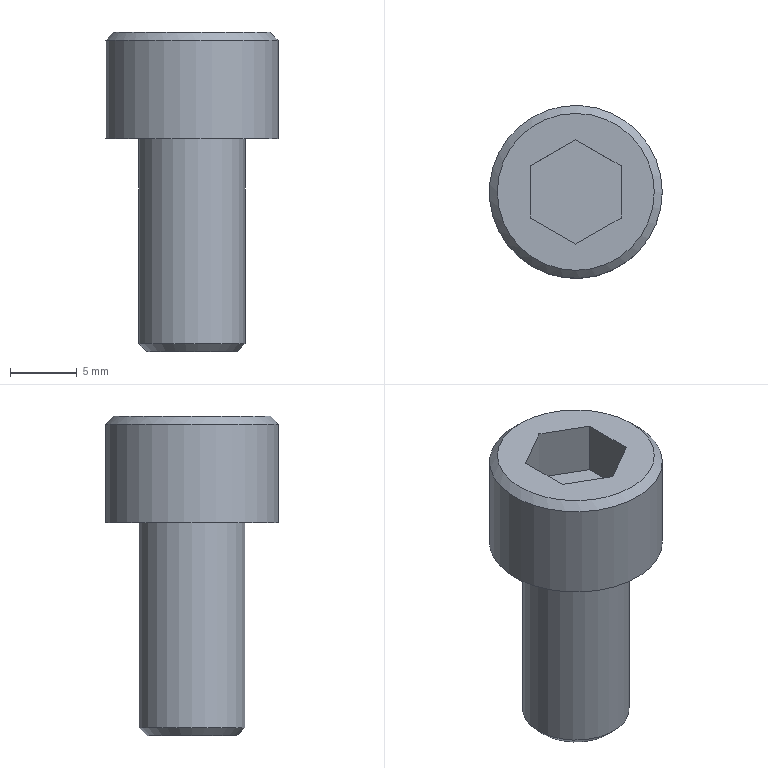Part | NX | features M8.00-50.00 2 | 1 solid | 14 faces | box 13 x 13 x 24 mm | volume 1695 mm3 | plane 10 | cylinder 2 | cone 2 | commonest cylinder face diameters 8 x1 13 x1
STEP:
#1=CARTESIAN_POINT('',(169.4,-50.,-42.));
#2=VERTEX_POINT('',#1);
#3=CARTESIAN_POINT('',(163.5,-50.,-42.));
#4=DIRECTION('',(0.,0.,1.));
#5=DIRECTION('',(1.,0.,0.));
#6=AXIS2_PLACEMENT_3D('',#3,#4,#5);
#7=CIRCLE('',#6,5.9);
#8=EDGE_CURVE('',#2,#2,#7,.T.);
#9=ORIENTED_EDGE('',*,*,#8,.T.);
#10=EDGE_LOOP('',(#9));
#11=FACE_BOUND('',#10,.T.);
#12=CARTESIAN_POINT('',(160.1,-48.037,-42.));
#13=VERTEX_POINT('',#12);
#14=CARTESIAN_POINT('',(160.1,-51.963,-42.));
#15=VERTEX_POINT('',#14);
#16=CARTESIAN_POINT('',(160.1,-48.037,-42.));
#17=DIRECTION('',(0.,-1.,0.));
#18=VECTOR('',#17,1000.);
#19=LINE('',#16,#18);
#20=EDGE_CURVE('',#13,#15,#19,.T.);
#21=ORIENTED_EDGE('',*,*,#20,.F.);
#22=CARTESIAN_POINT('',(163.5,-46.074,-42.));
#23=VERTEX_POINT('',#22);
#24=CARTESIAN_POINT('',(163.5,-46.074,-42.));
#25=DIRECTION('',(-0.866,-0.5,0.));
#26=VECTOR('',#25,1000.);
#27=LINE('',#24,#26);
#28=EDGE_CURVE('',#23,#13,#27,.T.);
#29=ORIENTED_EDGE('',*,*,#28,.F.);
#30=CARTESIAN_POINT('',(166.9,-48.037,-42.));
#31=VERTEX_POINT('',#30);
#32=CARTESIAN_POINT('',(166.9,-48.037,-42.));
#33=DIRECTION('',(-0.866,0.5,0.));
#34=VECTOR('',#33,1000.);
#35=LINE('',#32,#34);
#36=EDGE_CURVE('',#31,#23,#35,.T.);
#37=ORIENTED_EDGE('',*,*,#36,.F.);
#38=CARTESIAN_POINT('',(166.9,-51.963,-42.));
#39=VERTEX_POINT('',#38);
#40=CARTESIAN_POINT('',(166.9,-51.963,-42.));
#41=DIRECTION('',(0.,1.,0.));
#42=VECTOR('',#41,1000.);
#43=LINE('',#40,#42);
#44=EDGE_CURVE('',#39,#31,#43,.T.);
#45=ORIENTED_EDGE('',*,*,#44,.F.);
#46=CARTESIAN_POINT('',(163.5,-53.926,-42.));
#47=VERTEX_POINT('',#46);
#48=CARTESIAN_POINT('',(163.5,-53.926,-42.));
#49=DIRECTION('',(0.866,0.5,0.));
#50=VECTOR('',#49,1000.);
#51=LINE('',#48,#50);
#52=EDGE_CURVE('',#47,#39,#51,.T.);
#53=ORIENTED_EDGE('',*,*,#52,.F.);
#54=CARTESIAN_POINT('',(160.1,-51.963,-42.));
#55=DIRECTION('',(0.866,-0.5,0.));
#56=VECTOR('',#55,1000.);
#57=LINE('',#54,#56);
#58=EDGE_CURVE('',#15,#47,#57,.T.);
#59=ORIENTED_EDGE('',*,*,#58,.F.);
#60=EDGE_LOOP('',(#21,#29,#37,#45,#53,#59));
#61=FACE_BOUND('',#60,.T.);
#62=CARTESIAN_POINT('',(163.5,-50.,-42.));
#63=DIRECTION('',(0.,0.,1.));
#64=DIRECTION('',(1.,0.,0.));
#65=AXIS2_PLACEMENT_3D('',#62,#63,#64);
#66=PLANE('',#65);
#67=ADVANCED_FACE('',(#11,#61),#66,.T.);
#68=CARTESIAN_POINT('',(167.5,-50.,-50.));
#69=VERTEX_POINT('',#68);
#70=CARTESIAN_POINT('',(163.5,-50.,-50.));
#71=DIRECTION('',(0.,0.,-1.));
#72=DIRECTION('',(1.,0.,0.));
#73=AXIS2_PLACEMENT_3D('',#70,#71,#72);
#74=CIRCLE('',#73,4.);
#75=EDGE_CURVE('',#69,#69,#74,.T.);
#76=ORIENTED_EDGE('',*,*,#75,.F.);
#77=EDGE_LOOP('',(#76));
#78=FACE_BOUND('',#77,.T.);
#79=CARTESIAN_POINT('',(170.,-50.,-50.));
#80=VERTEX_POINT('',#79);
#81=CARTESIAN_POINT('',(163.5,-50.,-50.));
#82=DIRECTION('',(0.,0.,1.));
#83=DIRECTION('',(1.,0.,0.));
#84=AXIS2_PLACEMENT_3D('',#81,#82,#83);
#85=CIRCLE('',#84,6.5);
#86=EDGE_CURVE('',#80,#80,#85,.T.);
#87=ORIENTED_EDGE('',*,*,#86,.F.);
#88=EDGE_LOOP('',(#87));
#89=FACE_BOUND('',#88,.T.);
#90=CARTESIAN_POINT('',(163.5,-50.,-50.));
#91=DIRECTION('',(0.,0.,-1.));
#92=DIRECTION('',(-1.,0.,0.));
#93=AXIS2_PLACEMENT_3D('',#90,#91,#92);
#94=PLANE('',#93);
#95=ADVANCED_FACE('',(#78,#89),#94,.T.);
#96=CARTESIAN_POINT('',(170.,-50.,-42.6));
#97=VERTEX_POINT('',#96);
#98=CARTESIAN_POINT('',(163.5,-50.,-42.6));
#99=DIRECTION('',(0.,0.,1.));
#100=DIRECTION('',(1.,0.,0.));
#101=AXIS2_PLACEMENT_3D('',#98,#99,#100);
#102=CIRCLE('',#101,6.5);
#103=EDGE_CURVE('',#97,#97,#102,.F.);
#104=ORIENTED_EDGE('',*,*,#103,.T.);
#105=EDGE_LOOP('',(#104));
#106=FACE_BOUND('',#105,.T.);
#107=ORIENTED_EDGE('',*,*,#86,.T.);
#108=EDGE_LOOP('',(#107));
#109=FACE_BOUND('',#108,.T.);
#110=CARTESIAN_POINT('',(163.5,-50.,-50.));
#111=DIRECTION('',(0.,0.,1.));
#112=DIRECTION('',(1.,0.,0.));
#113=AXIS2_PLACEMENT_3D('',#110,#111,#112);
#114=CYLINDRICAL_SURFACE('',#113,6.5);
#115=ADVANCED_FACE('',(#106,#109),#114,.T.);
#116=CARTESIAN_POINT('',(160.1,-50.,-66.));
#117=VERTEX_POINT('',#116);
#118=CARTESIAN_POINT('',(163.5,-50.,-66.));
#119=DIRECTION('',(0.,0.,-1.));
#120=DIRECTION('',(-1.,0.,0.));
#121=AXIS2_PLACEMENT_3D('',#118,#119,#120);
#122=CIRCLE('',#121,3.4);
#123=EDGE_CURVE('',#117,#117,#122,.T.);
#124=ORIENTED_EDGE('',*,*,#123,.T.);
#125=EDGE_LOOP('',(#124));
#126=FACE_BOUND('',#125,.T.);
#127=CARTESIAN_POINT('',(163.5,-50.,-66.));
#128=DIRECTION('',(0.,0.,-1.));
#129=DIRECTION('',(-1.,0.,0.));
#130=AXIS2_PLACEMENT_3D('',#127,#128,#129);
#131=PLANE('',#130);
#132=ADVANCED_FACE('',(#126),#131,.T.);
#133=CARTESIAN_POINT('',(159.5,-50.,-65.4));
#134=VERTEX_POINT('',#133);
#135=CARTESIAN_POINT('',(163.5,-50.,-65.4));
#136=DIRECTION('',(0.,0.,-1.));
#137=DIRECTION('',(-1.,0.,0.));
#138=AXIS2_PLACEMENT_3D('',#135,#136,#137);
#139=CIRCLE('',#138,4.);
#140=EDGE_CURVE('',#134,#134,#139,.F.);
#141=ORIENTED_EDGE('',*,*,#140,.T.);
#142=EDGE_LOOP('',(#141));
#143=FACE_BOUND('',#142,.T.);
#144=ORIENTED_EDGE('',*,*,#75,.T.);
#145=EDGE_LOOP('',(#144));
#146=FACE_BOUND('',#145,.T.);
#147=CARTESIAN_POINT('',(163.5,-50.,-24.5));
#148=DIRECTION('',(0.,0.,-1.));
#149=DIRECTION('',(1.,0.,0.));
#150=AXIS2_PLACEMENT_3D('',#147,#148,#149);
#151=CYLINDRICAL_SURFACE('',#150,4.);
#152=ADVANCED_FACE('',(#143,#146),#151,.T.);
#153=ORIENTED_EDGE('',*,*,#58,.T.);
#154=CARTESIAN_POINT('',(163.5,-53.926,-46.));
#155=VERTEX_POINT('',#154);
#156=CARTESIAN_POINT('',(163.5,-53.926,-46.));
#157=DIRECTION('',(0.,0.,1.));
#158=VECTOR('',#157,1000.);
#159=LINE('',#156,#158);
#160=EDGE_CURVE('',#47,#155,#159,.F.);
#161=ORIENTED_EDGE('',*,*,#160,.T.);
#162=CARTESIAN_POINT('',(160.1,-51.963,-46.));
#163=VERTEX_POINT('',#162);
#164=CARTESIAN_POINT('',(160.1,-51.963,-46.));
#165=DIRECTION('',(0.866,-0.5,0.));
#166=VECTOR('',#165,1000.);
#167=LINE('',#164,#166);
#168=EDGE_CURVE('',#155,#163,#167,.F.);
#169=ORIENTED_EDGE('',*,*,#168,.T.);
#170=CARTESIAN_POINT('',(160.1,-51.963,-46.));
#171=DIRECTION('',(0.,0.,1.));
#172=VECTOR('',#171,1000.);
#173=LINE('',#170,#172);
#174=EDGE_CURVE('',#15,#163,#173,.F.);
#175=ORIENTED_EDGE('',*,*,#174,.F.);
#176=EDGE_LOOP('',(#153,#161,#169,#175));
#177=FACE_BOUND('',#176,.T.);
#178=CARTESIAN_POINT('',(161.8,-52.944,-44.));
#179=DIRECTION('',(-0.5,-0.866,0.));
#180=DIRECTION('',(0.866,-0.5,0.));
#181=AXIS2_PLACEMENT_3D('',#178,#179,#180);
#182=PLANE('',#181);
#183=ADVANCED_FACE('',(#177),#182,.F.);
#184=ORIENTED_EDGE('',*,*,#20,.T.);
#185=ORIENTED_EDGE('',*,*,#174,.T.);
#186=CARTESIAN_POINT('',(160.1,-48.037,-46.));
#187=VERTEX_POINT('',#186);
#188=CARTESIAN_POINT('',(160.1,-48.037,-46.));
#189=DIRECTION('',(0.,-1.,0.));
#190=VECTOR('',#189,1000.);
#191=LINE('',#188,#190);
#192=EDGE_CURVE('',#163,#187,#191,.F.);
#193=ORIENTED_EDGE('',*,*,#192,.T.);
#194=CARTESIAN_POINT('',(160.1,-48.037,-46.));
#195=DIRECTION('',(0.,0.,1.));
#196=VECTOR('',#195,1000.);
#197=LINE('',#194,#196);
#198=EDGE_CURVE('',#13,#187,#197,.F.);
#199=ORIENTED_EDGE('',*,*,#198,.F.);
#200=EDGE_LOOP('',(#184,#185,#193,#199));
#201=FACE_BOUND('',#200,.T.);
#202=CARTESIAN_POINT('',(160.1,-50.,-44.));
#203=DIRECTION('',(-1.,0.,0.));
#204=DIRECTION('',(0.,0.,1.));
#205=AXIS2_PLACEMENT_3D('',#202,#203,#204);
#206=PLANE('',#205);
#207=ADVANCED_FACE('',(#201),#206,.F.);
#208=ORIENTED_EDGE('',*,*,#28,.T.);
#209=ORIENTED_EDGE('',*,*,#198,.T.);
#210=CARTESIAN_POINT('',(163.5,-46.074,-46.));
#211=VERTEX_POINT('',#210);
#212=CARTESIAN_POINT('',(163.5,-46.074,-46.));
#213=DIRECTION('',(-0.866,-0.5,0.));
#214=VECTOR('',#213,1000.);
#215=LINE('',#212,#214);
#216=EDGE_CURVE('',#187,#211,#215,.F.);
#217=ORIENTED_EDGE('',*,*,#216,.T.);
#218=CARTESIAN_POINT('',(163.5,-46.074,-46.));
#219=DIRECTION('',(0.,0.,1.));
#220=VECTOR('',#219,1000.);
#221=LINE('',#218,#220);
#222=EDGE_CURVE('',#23,#211,#221,.F.);
#223=ORIENTED_EDGE('',*,*,#222,.F.);
#224=EDGE_LOOP('',(#208,#209,#217,#223));
#225=FACE_BOUND('',#224,.T.);
#226=CARTESIAN_POINT('',(161.8,-47.056,-44.));
#227=DIRECTION('',(-0.5,0.866,0.));
#228=DIRECTION('',(-0.866,-0.5,0.));
#229=AXIS2_PLACEMENT_3D('',#226,#227,#228);
#230=PLANE('',#229);
#231=ADVANCED_FACE('',(#225),#230,.F.);
#232=ORIENTED_EDGE('',*,*,#36,.T.);
#233=ORIENTED_EDGE('',*,*,#222,.T.);
#234=CARTESIAN_POINT('',(166.9,-48.037,-46.));
#235=VERTEX_POINT('',#234);
#236=CARTESIAN_POINT('',(166.9,-48.037,-46.));
#237=DIRECTION('',(-0.866,0.5,0.));
#238=VECTOR('',#237,1000.);
#239=LINE('',#236,#238);
#240=EDGE_CURVE('',#211,#235,#239,.F.);
#241=ORIENTED_EDGE('',*,*,#240,.T.);
#242=CARTESIAN_POINT('',(166.9,-48.037,-46.));
#243=DIRECTION('',(0.,0.,1.));
#244=VECTOR('',#243,1000.);
#245=LINE('',#242,#244);
#246=EDGE_CURVE('',#31,#235,#245,.F.);
#247=ORIENTED_EDGE('',*,*,#246,.F.);
#248=EDGE_LOOP('',(#232,#233,#241,#247));
#249=FACE_BOUND('',#248,.T.);
#250=CARTESIAN_POINT('',(165.2,-47.056,-44.));
#251=DIRECTION('',(0.5,0.866,0.));
#252=DIRECTION('',(-0.866,0.5,0.));
#253=AXIS2_PLACEMENT_3D('',#250,#251,#252);
#254=PLANE('',#253);
#255=ADVANCED_FACE('',(#249),#254,.F.);
#256=ORIENTED_EDGE('',*,*,#44,.T.);
#257=ORIENTED_EDGE('',*,*,#246,.T.);
#258=CARTESIAN_POINT('',(166.9,-51.963,-46.));
#259=VERTEX_POINT('',#258);
#260=CARTESIAN_POINT('',(166.9,-51.963,-46.));
#261=DIRECTION('',(0.,1.,0.));
#262=VECTOR('',#261,1000.);
#263=LINE('',#260,#262);
#264=EDGE_CURVE('',#235,#259,#263,.F.);
#265=ORIENTED_EDGE('',*,*,#264,.T.);
#266=CARTESIAN_POINT('',(166.9,-51.963,-46.));
#267=DIRECTION('',(0.,0.,1.));
#268=VECTOR('',#267,1000.);
#269=LINE('',#266,#268);
#270=EDGE_CURVE('',#39,#259,#269,.F.);
#271=ORIENTED_EDGE('',*,*,#270,.F.);
#272=EDGE_LOOP('',(#256,#257,#265,#271));
#273=FACE_BOUND('',#272,.T.);
#274=CARTESIAN_POINT('',(166.9,-50.,-44.));
#275=DIRECTION('',(1.,0.,0.));
#276=DIRECTION('',(0.,0.,-1.));
#277=AXIS2_PLACEMENT_3D('',#274,#275,#276);
#278=PLANE('',#277);
#279=ADVANCED_FACE('',(#273),#278,.F.);
#280=ORIENTED_EDGE('',*,*,#52,.T.);
#281=ORIENTED_EDGE('',*,*,#270,.T.);
#282=CARTESIAN_POINT('',(163.5,-53.926,-46.));
#283=DIRECTION('',(0.866,0.5,0.));
#284=VECTOR('',#283,1000.);
#285=LINE('',#282,#284);
#286=EDGE_CURVE('',#259,#155,#285,.F.);
#287=ORIENTED_EDGE('',*,*,#286,.T.);
#288=ORIENTED_EDGE('',*,*,#160,.F.);
#289=EDGE_LOOP('',(#280,#281,#287,#288));
#290=FACE_BOUND('',#289,.T.);
#291=CARTESIAN_POINT('',(165.2,-52.944,-44.));
#292=DIRECTION('',(0.5,-0.866,0.));
#293=DIRECTION('',(0.866,0.5,0.));
#294=AXIS2_PLACEMENT_3D('',#291,#292,#293);
#295=PLANE('',#294);
#296=ADVANCED_FACE('',(#290),#295,.F.);
#297=ORIENTED_EDGE('',*,*,#286,.F.);
#298=ORIENTED_EDGE('',*,*,#264,.F.);
#299=ORIENTED_EDGE('',*,*,#240,.F.);
#300=ORIENTED_EDGE('',*,*,#216,.F.);
#301=ORIENTED_EDGE('',*,*,#192,.F.);
#302=ORIENTED_EDGE('',*,*,#168,.F.);
#303=EDGE_LOOP('',(#297,#298,#299,#300,#301,#302));
#304=FACE_BOUND('',#303,.T.);
#305=CARTESIAN_POINT('',(163.5,-50.,-46.));
#306=DIRECTION('',(0.,0.,-1.));
#307=DIRECTION('',(-1.,0.,0.));
#308=AXIS2_PLACEMENT_3D('',#305,#306,#307);
#309=PLANE('',#308);
#310=ADVANCED_FACE('',(#304),#309,.F.);
#311=ORIENTED_EDGE('',*,*,#123,.F.);
#312=EDGE_LOOP('',(#311));
#313=FACE_BOUND('',#312,.T.);
#314=ORIENTED_EDGE('',*,*,#140,.F.);
#315=EDGE_LOOP('',(#314));
#316=FACE_BOUND('',#315,.T.);
#317=CARTESIAN_POINT('',(163.5,-50.,-65.4));
#318=DIRECTION('',(0.,0.,1.));
#319=DIRECTION('',(1.,0.,0.));
#320=AXIS2_PLACEMENT_3D('',#317,#318,#319);
#321=CONICAL_SURFACE('',#320,4.,0.7854);
#322=ADVANCED_FACE('',(#313,#316),#321,.T.);
#323=ORIENTED_EDGE('',*,*,#8,.F.);
#324=EDGE_LOOP('',(#323));
#325=FACE_BOUND('',#324,.T.);
#326=ORIENTED_EDGE('',*,*,#103,.F.);
#327=EDGE_LOOP('',(#326));
#328=FACE_BOUND('',#327,.T.);
#329=CARTESIAN_POINT('',(163.5,-50.,-42.6));
#330=DIRECTION('',(0.,0.,-1.));
#331=DIRECTION('',(-1.,0.,0.));
#332=AXIS2_PLACEMENT_3D('',#329,#330,#331);
#333=CONICAL_SURFACE('',#332,6.5,0.7854);
#334=ADVANCED_FACE('',(#325,#328),#333,.T.);
#335=CLOSED_SHELL('',(#67,#95,#115,#132,#152,#183,#207,#231,#255,#279,#296,#310,#322,#334));
#336=MANIFOLD_SOLID_BREP('',#335);
#337=(LENGTH_UNIT()NAMED_UNIT(*)SI_UNIT(.MILLI.,.METRE.));
#338=UNCERTAINTY_MEASURE_WITH_UNIT(LENGTH_MEASURE(0.00001),#337,'','');
#339=(NAMED_UNIT(*)PLANE_ANGLE_UNIT()SI_UNIT($,.RADIAN.));
#340=(NAMED_UNIT(*)SI_UNIT($,.STERADIAN.)SOLID_ANGLE_UNIT());
#341=(GEOMETRIC_REPRESENTATION_CONTEXT(3)GLOBAL_UNCERTAINTY_ASSIGNED_CONTEXT((#338))GLOBAL_UNIT_ASSIGNED_CONTEXT((#337,#339,#340))REPRESENTATION_CONTEXT('',''));
#342=ADVANCED_BREP_SHAPE_REPRESENTATION('',(#336),#341);